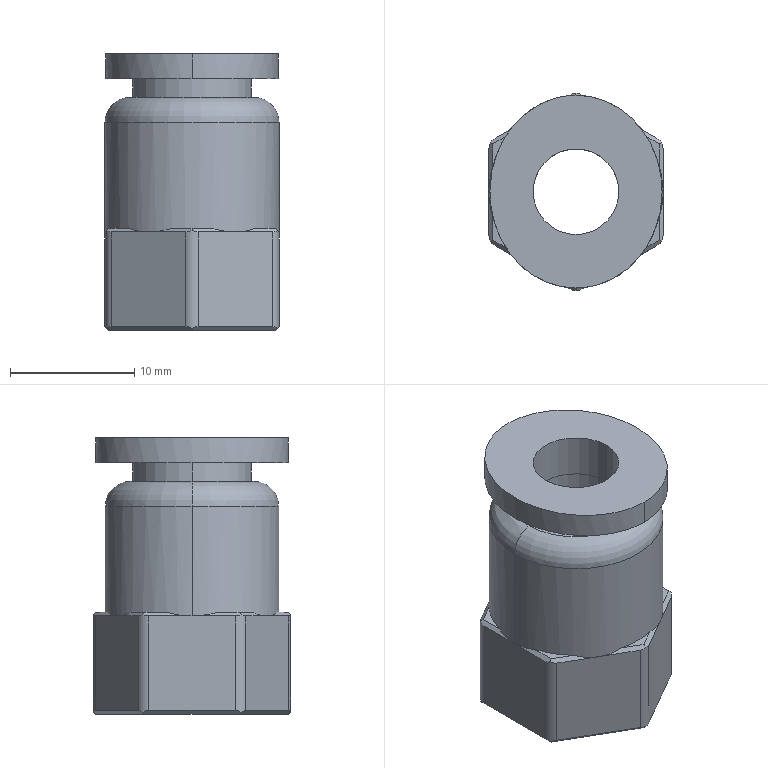Part | SolidWorks | features BaseBody 2 | 2 solids | 86 faces | box 14 x 15.856 x 22.23 mm | volume 2429 mm3 | cylinder 38 | plane 38 | spline 4 | torus 4 | cone 2 | commonest cylinder face diameters 7.779 x12 9.17 x12 2 x6 6.9 x4 9.5 x2 14 x2